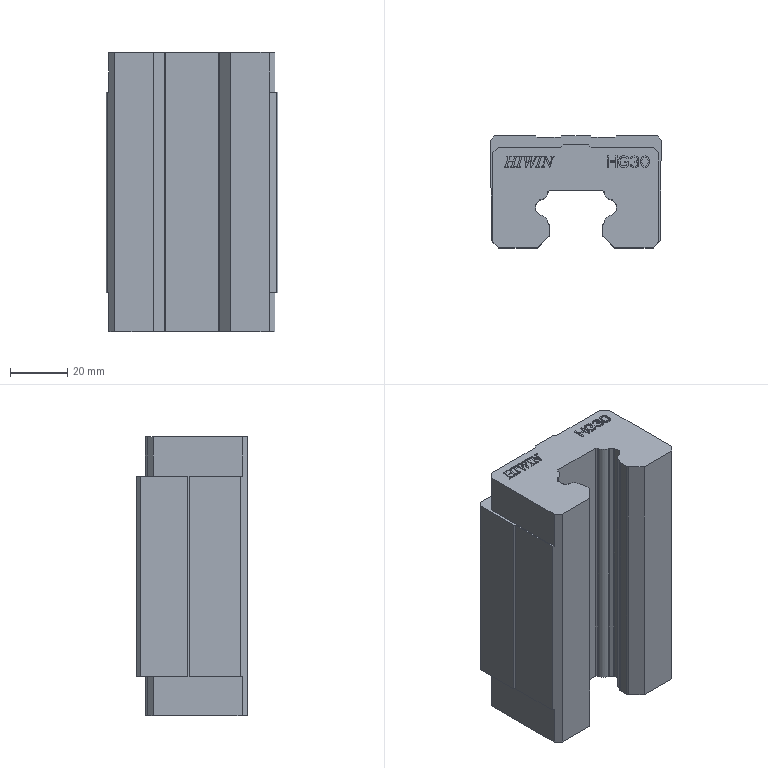Part | SolidWorks | features BaseBody 1 | 1 solid | 390 faces | box 60 x 39 x 97.7 mm | volume 170717 mm3 | plane 302 | spline 60 | cylinder 28 | commonest cylinder face diameters 1.2 x12 8 x8 1.6 x4 5.66 x4